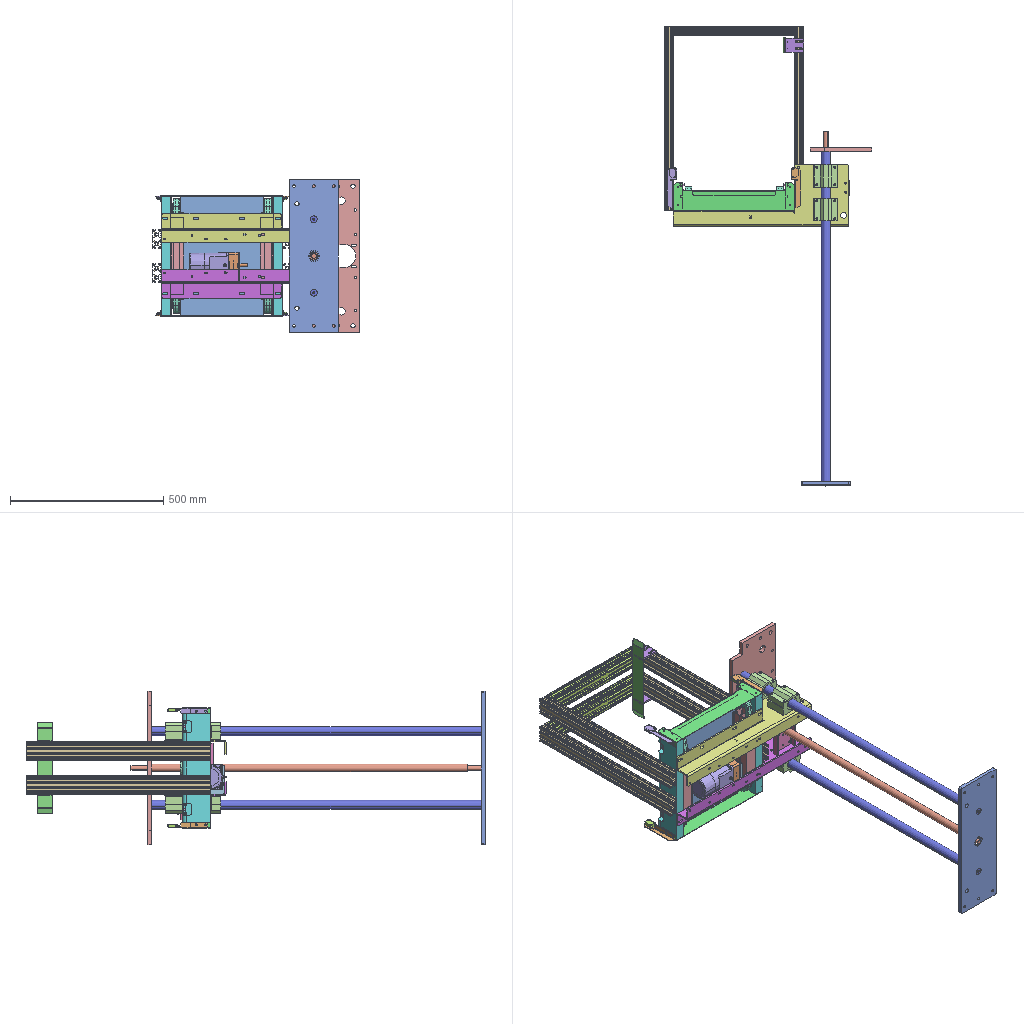Assembly | SolidWorks | 29 different items | 48 placed | box 677 x 1499 x 500 mm
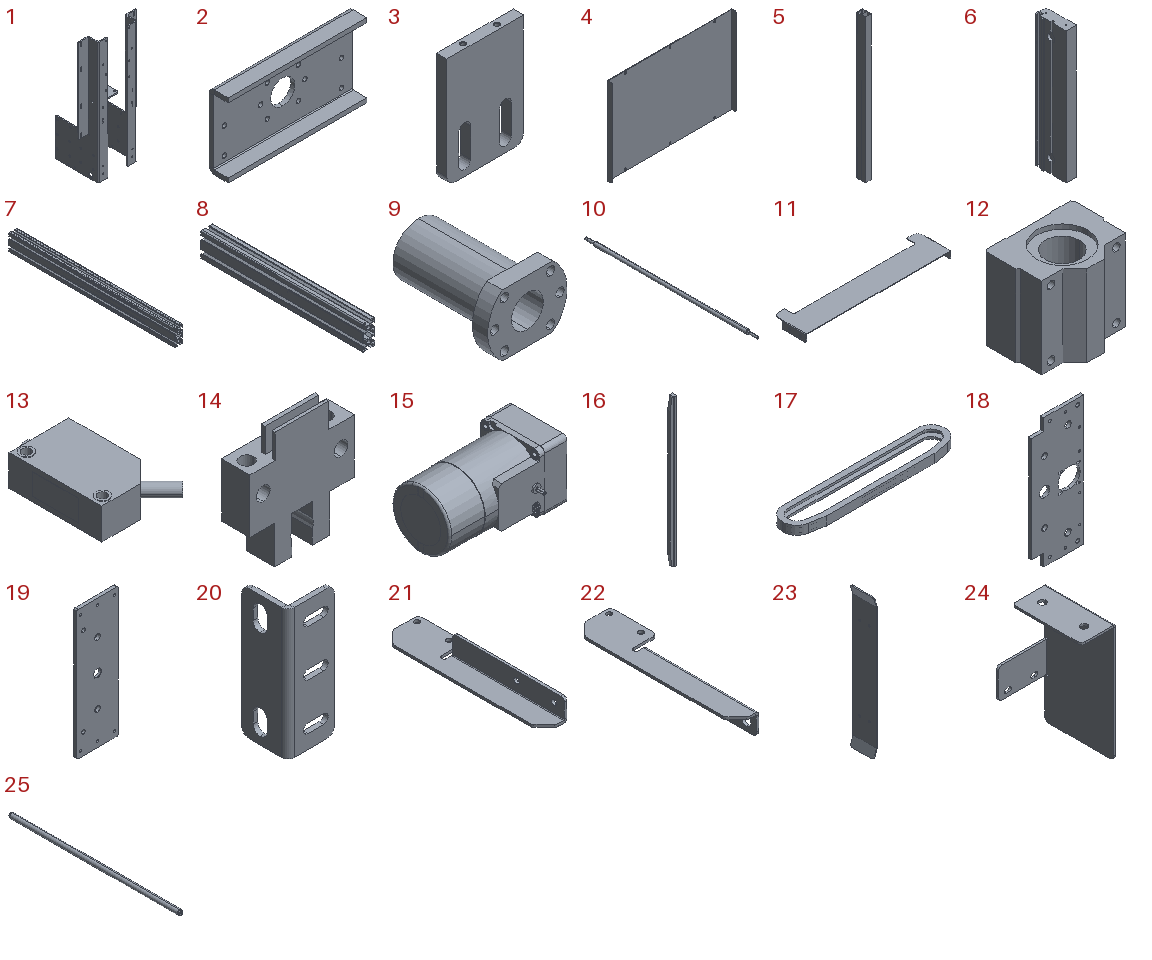Parts list (item | name | quantity | size | volume | features):
1 | - | x1 | 274 x 202 x 570 mm | 975509 mm3 | features HoleWzd 9, FlatPattern 3, ICE 3, EdgeFlange 2, Fillet 2, SMBaseFlange 2, SheetMetal 2, TabAndSlotFeature 2, Cut 1, DeleteBody 1, MirrorSolid 1
2 | - | x1 | 160 x 22 x 85 mm | 88540 mm3 | features HoleWzd 2, CirPattern 1, EdgeFlange 1, FlatPattern 1, SMBaseFlange 1, SheetMetal 1
3 | - | x2 | 45 x 6 x 65 mm | 15460 mm3 | features Extrusion 1, Fillet 1, HoleWzd 1, ICE 1
4 | - | x1 | 390 x 15 x 272 mm | 169539 mm3 | features ICE 2, BreakCorner 1, EdgeFlange 1, FlatPattern 1, SMBaseFlange 1, SheetMetal 1
5 | - | x2 | 43 x 64.5 x 1060 mm | 529141 mm3 | features Extrusion 1
6 | - | x2 | 34.5 x 90 x 390 mm | 934909 mm3 | features ICE 3, HoleWzd 2, MirrorPattern 2, Extrusion 1
7 | - | x4 | 30 x 600 x 60 mm | 300183 mm3 | features WeldMemberFeat 1, WeldmentFeature 1
8 | - | x2 | 30 x 395 x 60 mm | 197620 mm3 | features WeldMemberFeat 1, WeldmentFeature 1
9 | - | x1 | 62 x 85 x 48 mm | 79345 mm3 | features CirPattern 1, Extrusion 1, HoleWzd 1, ICE 1
10 | - | x1 | 25 x 1157 x 25 mm | 530644 mm3 | features Revolution 1
11 | - | x2 | 398 x 90 x 20 mm | 44260 mm3 | features Fillet 3, EdgeFlange 1, FlatPattern 1, HoleWzd 1, ICE 1, SMBaseFlange 1, SheetMetal 1
12 | - | x4 | 78 x 59.5 x 72 mm | 221969 mm3 | features MBimport 1
13 | - | x4 | 24.985 x 38.085 x 10.8 mm | 6244 mm3 | features BaseBody 1
14 | - | x1 | 25.5 x 6.9 x 28.5 mm | 2565 mm3 | features ICE 4, HoleWzd 2, Emboss 1, Extrusion 1
15 | - | x1 | 190 x 92 x 80 mm | 778868 mm3 | features BaseBody 2
16 | - | x2 | 14 x 11 x 390 mm | 45277 mm3 | features Chamfer 1, Extrusion 1, Fillet 1
17 | - | x2 | 375 x 70.699 x 20 mm | 102724 mm3 | features Extrusion 1, ICE 1
18 | - | x1 | 200 x 12 x 500 mm | 1034176 mm3 | features ICE 7, HoleWzd 3, Fillet 2, Extrusion 1
19 | - | x1 | 160 x 12 x 500 mm | 931309 mm3 | features ICE 3, Extrusion 1, Fillet 1, HoleWzd 1
20 | - | x1 | 30 x 30 x 84 mm | 12475 mm3 | features HoleWzd 2, EdgeFlange 1, Fillet 1, FlatPattern 1, SMBaseFlange 1, SheetMetal 1
21 | - | x2 | 30 x 130 x 17 mm | 7736 mm3 | features HoleWzd 2, EdgeFlange 1, Fillet 1, FlatPattern 1, SMBaseFlange 1, SheetMetal 1
22 | - | x2 | 30 x 130 x 17 mm | 7638 mm3 | features HoleWzd 2, EdgeFlange 1, Fillet 1, FlatPattern 1, SMBaseFlange 1, SheetMetal 1
23 | - | x1 | 7.789 x 50 x 299.041 mm | 29866 mm3 | features EdgeFlange 1, Fillet 1, FlatPattern 1, HoleWzd 1, MirrorPattern 1, SMBaseFlange 1, SheetMetal 1
24 | - | x1 | 36.5 x 50 x 85 mm | 9132 mm3 | features EdgeFlange 2, HoleWzd 2, Fillet 1, FlatPattern 1, SMBaseFlange 1, SheetMetal 1
25 | - | x2 | 30 x 1095 x 30 mm | 765991 mm3 | features HoleWzd 2, ICE 2, Extrusion 1
26 | XS2413028B-Lever Cylinder Base | x1 | - | - | -
27 | XS2413035B-Bin Clamping Cylinder Mounting Plate | x1 | - | - | -
28 | XS2416004B-Lifting Motor | x1 | - | - | -
29 | XS2416006B-BLC Lever Cylinder | x1 | - | - | -
Mates (type | each side: item.copy, entity, surface, feature):
Concentric | 18.1 face cylinder Cut-Extrude1 | 19.1 face cylinder Cut-Extrude2
Concentric | 18.1 face cylinder Cut-Extrude1 | 19.1 face cylinder Cut-Extrude1
DistanceDim | 19.1 face plane Boss-Extrude1 | 18.1 face plane Boss-Extrude1
Coincident | 18.1 face plane Boss-Extrude1 | 25.1 face plane Boss-Extrude1
Concentric | 18.1 face cylinder Cut-Extrude1 | 25.1 face cylinder Boss-Extrude1
Coincident | 18.1 face plane Boss-Extrude1 | 25.2 face plane Boss-Extrude1
Concentric | 18.1 face cylinder Cut-Extrude1 | 25.2 face cylinder Boss-Extrude1
Concentric | 18.1 face cylinder Cut-Extrude1 | 10.1 face cylinder Revolve1
Concentric | 25.1 face cylinder Boss-Extrude1 | 12.1 face cylinder LMW01-d30.stp
Concentric | 25.1 face cylinder Boss-Extrude1 | 12.2 face cylinder LMW01-d30.stp
Concentric | 25.2 face cylinder Boss-Extrude1 | 12.3 face cylinder LMW01-d30.stp
Concentric | 25.2 face cylinder Boss-Extrude1 | 12.4 face cylinder LMW01-d30.stp
Coincident | 1.1 face plane Mirror1 | 12.2 face plane LMW01-d30.stp
Concentric | 1.1 face cylinder Mirror1 | 12.1 face cylinder LMW01-d30.stp
Concentric | 1.1 face cylinder Mirror1 | 12.2 face cylinder LMW01-d30.stp
Parallel | 18.1 face plane Boss-Extrude1 | 1.1 face plane Mirror1
Coincident | 1.1 face plane Base-Flange1 | 12.3 face plane LMW01-d30.stp
Coincident | 1.1 face plane Base-Flange1 | 12.4 face plane LMW01-d30.stp
Concentric | 1.1 face cylinder Ø8.0 (8) Diameter Hole1 | 12.3 face cylinder LMW01-d30.stp
Concentric | 1.1 face cylinder Ø8.0 (8) Diameter Hole1 | 12.4 face cylinder LMW01-d30.stp
Concentric | 10.1 face cylinder Revolve1 | 2.1 face cylinder Base-Flange1
Concentric | 9.1 face cylinder Boss-Extrude2 | 10.1 face cylinder Revolve1
Coincident | 9.1 face plane Boss-Extrude1 | 2.1 face plane Base-Flange1
Concentric | 9.1 face cylinder CirPattern1 | 2.1 face cylinder CirPattern1
Parallel | 1.1 face plane Mirror1 | 2.1 face plane Edge-Flange1
Coincident | 20.1 face plane Base-Flange1 | 2.1 face plane Base-Flange1
Coincident | 20.1 face plane Edge-Flange1 | 1.1 face plane Mirror1
Concentric | 20.1 face cylinder Ø9.0 (9) Diameter slot1 | 1.1 face cylinder Mirror1
Coincident | 24.1 face plane Edge-Flange1 | 1.1 face plane Base-Flange1
Concentric | 24.1 face cylinder M6 Tapped Hole1 | 1.1 face cylinder Ø6.8 (6.8) Diameter Hole1 | 2 times
Coincident | 14.1 face plane Boss-Extrude1 | 24.1 face plane Edge-Flange2
Concentric | 14.1 face cylinder M3 Clearance Hole1 | 24.1 face cylinder Ø3.0 (3) Diameter slot1 | 2 times
Concentric | 13.1 face cylinder Imported1 | 21.1 face cylinder Ø4.0 (4) Diameter Hole1 | 2 times
Concentric | 22.1 face cylinder Ø4.0 (4) Diameter Hole1 | 13.2 face cylinder Imported1 | 2 times
Coincident | 1.1 face plane Mirror1 | 6.1 face plane Boss-Extrude1 | 2 times
Coincident | 6.1 face plane Boss-Extrude1 | 7.1 face plane Aluminum profile 30 X 60L X R2.5(1) | 2 times
Coincident | 1.1 face plane Mirror1 | 7.1 face plane Aluminum profile 30 X 60L X R2.5(1)
Width | 18.1 face plane Boss-Extrude1 | 18.1 face plane Boss-Extrude1 | 6.1 face plane Boss-Extrude1 | 6.1 face plane Boss-Extrude1
Coincident | 1.1 face plane Base-Flange1 | 7.2 face plane Aluminum profile 30 X 60L X R2.5(1)
Coincident | 6.1 face plane Boss-Extrude1 | 7.2 face plane Aluminum profile 30 X 60L X R2.5(1)
Coincident | 7.1 face plane Aluminum profile 30 X 60L X R2.5(1) | 7.2 face plane Aluminum profile 30 X 60L X R2.5(1)
Coincident | 7.2 face plane Aluminum profile 30 X 60L X R2.5(1) | 3.1 face plane Boss-Extrude1
Coincident | 7.1 face plane Aluminum profile 30 X 60L X R2.5(1) | 3.2 face plane Boss-Extrude1 | 2 times
Coincident | 3.1 face plane Boss-Extrude1 | 3.2 face plane Boss-Extrude1
Coincident | 23.1 face plane Base-Flange1 | 3.2 face plane Boss-Extrude1
Concentric | 23.1 face cylinder Ø4.2 (4.2) Diameter Hole1 | 3.2 face cylinder M3 Tapped Hole1
Concentric | 23.1 face cylinder Mirror1 | 3.1 face cylinder M3 Tapped Hole1
DistanceDim | 7.2 face plane Aluminum profile 30 X 60L X R2.5(1) | 3.1 face plane Boss-Extrude1
Coincident | 1.1 face plane Mirror1 | 6.2 face plane Boss-Extrude1
Coincident | 6.1 face plane Boss-Extrude1 | 6.2 face plane Boss-Extrude1
DistanceDim | 6.1 face plane Boss-Extrude1 | 6.2 face plane Boss-Extrude1
Coincident | 6.1 face plane Boss-Extrude1 | 11.1 face plane Edge-Flange1 | 2 times
Coincident | 6.1 face plane Boss-Extrude1 | 11.1 face plane Base-Flange1
Coincident | 6.1 face plane Boss-Extrude1 | 11.2 face plane Base-Flange1
Coincident | 6.1 face plane Boss-Extrude1 | 11.2 face plane Edge-Flange1 | 2 times
Coincident | 22.1 face plane Edge-Flange4 | 11.2 face plane Edge-Flange1
Concentric | 22.1 face cylinder Ø7.0 (7) Diameter Hole1 | 11.2 face cylinder Ø6.5 (6.5) Diameter Hole1 | 2 times
Coincident | 21.1 face plane Edge-Flange4 | 11.2 face plane Edge-Flange1
Concentric | 21.1 face cylinder Ø4.2 (4.2) Diameter Hole1 | 11.2 face cylinder Ø6.5 (6.5) Diameter Hole1 | 2 times
Coincident | 21.2 face plane Edge-Flange4 | 11.1 face plane Edge-Flange1
Coincident | 21.2 face plane Base-Flange1 | 13.3 face plane Imported1
Concentric | 21.2 face cylinder Ø4.2 (4.2) Diameter Hole1 | 11.1 face cylinder Ø6.5 (6.5) Diameter Hole1 | 2 times
Concentric | 21.2 face cylinder Ø4.0 (4) Diameter Hole1 | 13.3 face cylinder Imported1 | 2 times
Coincident | 13.1 face plane Imported1 | 21.1 face plane Base-Flange1
Coincident | 22.1 face plane Base-Flange1 | 13.2 face plane Imported1
Concentric | 22.2 face cylinder Ø4.0 (4) Diameter Hole1 | 13.4 face cylinder Imported1 | 2 times
Coincident | 22.2 face plane Base-Flange1 | 13.4 face plane Imported1
Coincident | 11.1 face plane Edge-Flange1 | 22.2 face plane Edge-Flange4
Concentric | 11.1 face cylinder Ø6.5 (6.5) Diameter Hole1 | 22.2 face cylinder Ø7.0 (7) Diameter Hole1 | 2 times
Coincident | 1.1 face plane Mirror1 | 5.1 face plane Boss-Extrude1
Coincident | 6.2 face plane Boss-Extrude1 | 5.1 face plane Boss-Extrude1
DistanceDim | 5.1 face plane Boss-Extrude1 | 6.2 face plane Boss-Extrude1
Coincident | 6.1 face plane Boss-Extrude1 | 5.2 face plane Boss-Extrude1 | 2 times
Coincident | 5.1 face plane Boss-Extrude1 | 5.2 face plane Boss-Extrude1
Coincident | 6.2 face plane Boss-Extrude1 | 7.3 face plane Aluminum profile 30 X 60L X R2.5(1)
Coincident | 7.1 face plane Aluminum profile 30 X 60L X R2.5(1) | 7.3 face plane Aluminum profile 30 X 60L X R2.5(1) | 2 times
Coincident | 6.2 face plane Boss-Extrude1 | 7.4 face plane Aluminum profile 30 X 60L X R2.5(1)
Coincident | 7.3 face plane Aluminum profile 30 X 60L X R2.5(1) | 7.4 face plane Aluminum profile 30 X 60L X R2.5(1)
Coincident | 7.2 face plane Aluminum profile 30 X 60L X R2.5(1) | 7.4 face plane Aluminum profile 30 X 60L X R2.5(1)
Coincident | 5.2 face plane Boss-Extrude1 | 4.1 face plane Base-Flange1 | 2 times
Coincident | 11.1 face plane Base-Flange1 | 4.1 face plane Edge-Flange1
Coincident | 7.1 face plane Aluminum profile 30 X 60L X R2.5(1) | 8.1 face plane Aluminum profile 30 X 60L X R2.5(1) | 3 times
Coincident | 7.2 face plane Aluminum profile 30 X 60L X R2.5(1) | 8.2 face plane Aluminum profile 30 X 60L X R2.5(1) | 3 times
Coincident | 6.1 face plane Boss-Extrude1 | 16.1 face plane Boss-Extrude1 | 3 times
Coincident | 6.2 face plane Boss-Extrude1 | 16.2 face plane Boss-Extrude1 | 3 times
Concentric | 6.2 face cylinder Cut-Extrude1 | 17.1 face cylinder Boss-Extrude1 | 2 times
Coincident | 5.1 face plane Boss-Extrude1 | 17.1 face plane Boss-Extrude1
Concentric | 6.2 face cylinder Cut-Extrude1 | 17.2 face cylinder Boss-Extrude1 | 2 times
Coincident | 5.2 face plane Boss-Extrude1 | 17.2 face plane Boss-Extrude1
Coincident | 1.1 face plane Base-Flange2 | 15.1 face plane MX8G30M-1-solid1
Concentric | 1.1 face cylinder Cut-Extrude1 | 15.1 face cylinder MX8G30M-1-solid1
Parallel | 1.1 face plane Base-Flange2 | 15.1 face plane MX8G30M-1-solid1
Coincident | 19.1 face plane Boss-Extrude1 | 10.1 face plane Revolve1